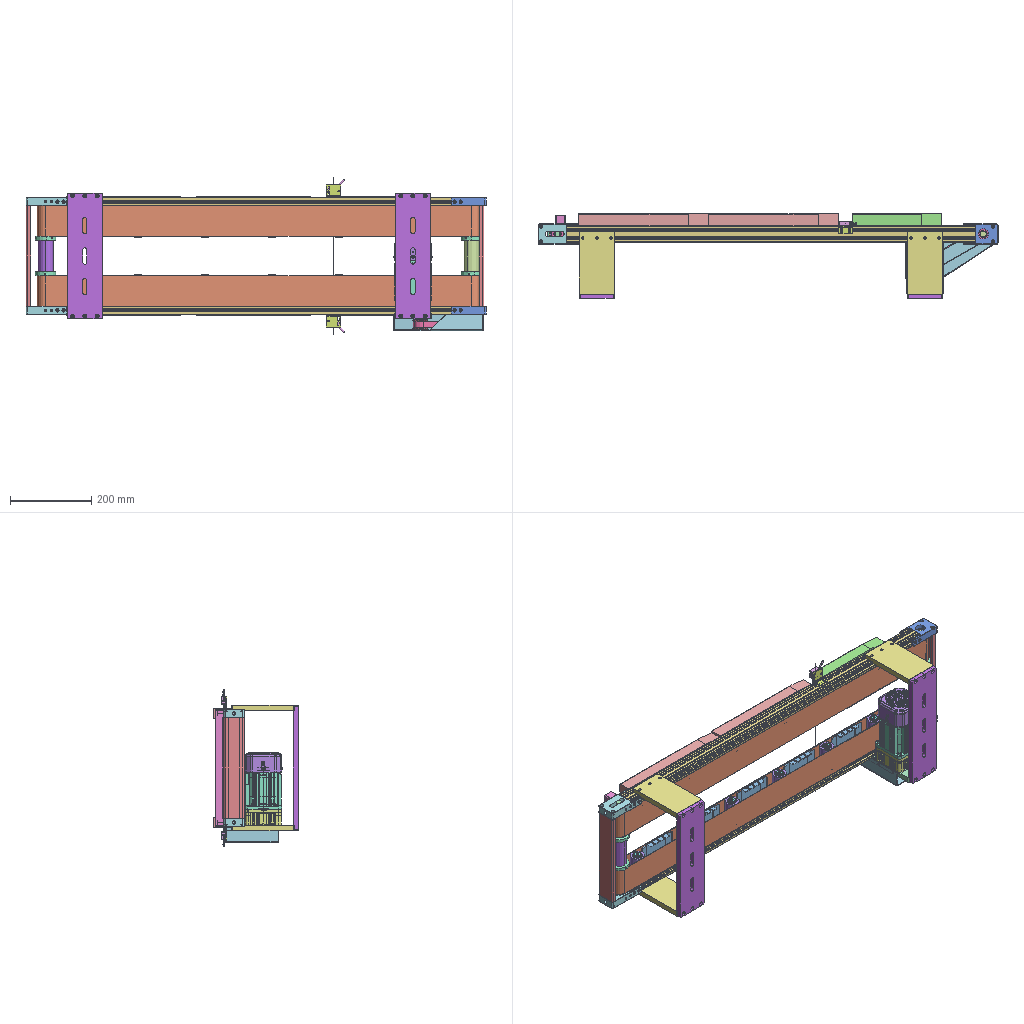Assembly | STEP file | 58 different items | 160 placed | box 1133 x 208 x 386 mm
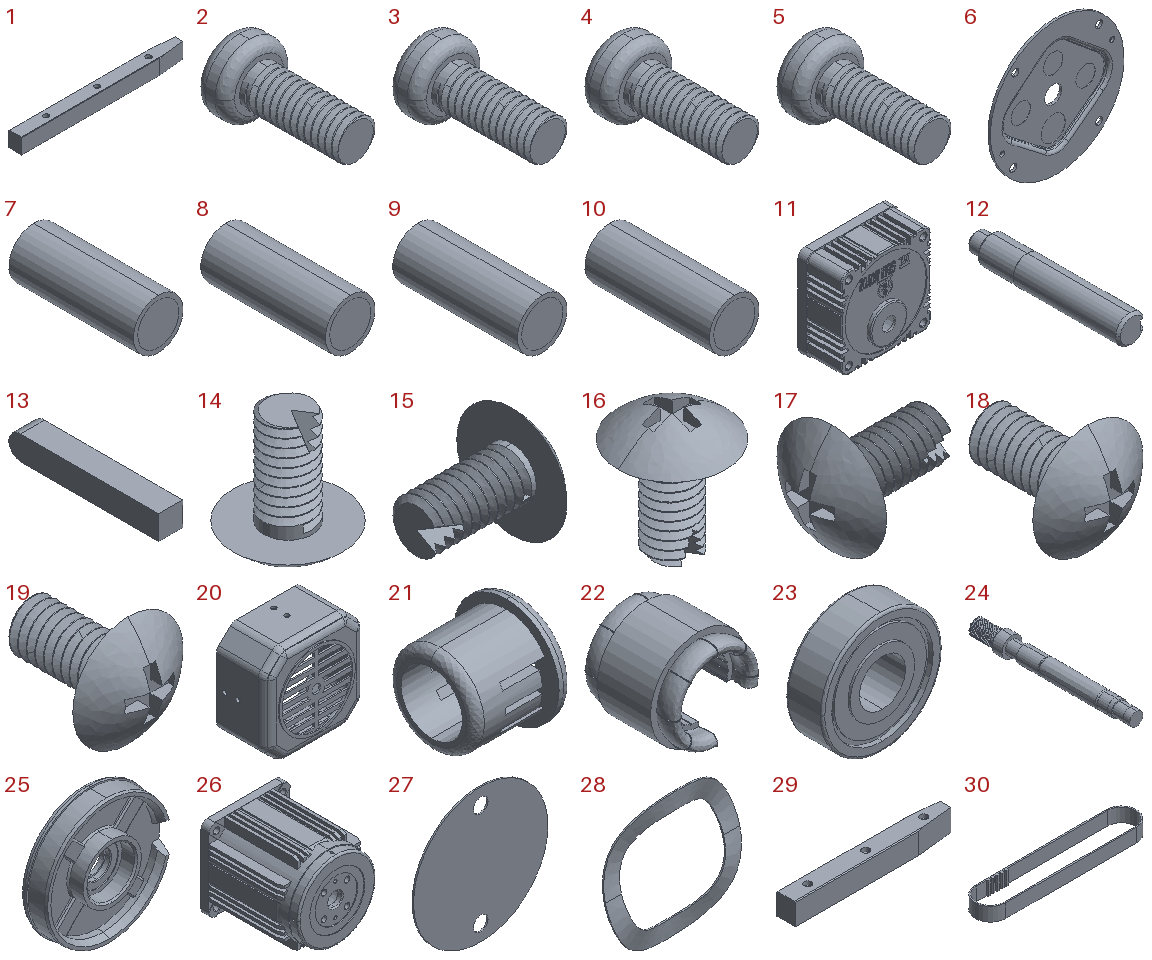Parts list (item | quantity | size | volume):
1 | x4 | 320 x 25 x 30 mm | 229201 mm3
2 | x1 | 7 x 13 x 7 mm | 186.803 mm3
3 | x1 | 7 x 13 x 7 mm | 186.803 mm3
4 | x1 | 7 x 13 x 7 mm | 186.803 mm3
5 | x1 | 7 x 13 x 7 mm | 186.803 mm3
6 | x1 | 82.5 x 4.2 x 82.5 mm | 8185 mm3
7 | x1 | 4 x 10 x 4 mm | 125.664 mm3
8 | x1 | 4 x 10 x 4 mm | 125.664 mm3
9 | x1 | 4 x 10 x 4 mm | 125.664 mm3
10 | x1 | 4 x 10 x 4 mm | 125.664 mm3
11 | x1 | 90 x 45 x 90 mm | 121396 mm3
12 | x1 | 12 x 67 x 12 mm | 6861 mm3
13 | x1 | 4 x 25 x 4 mm | 393.133 mm3
14 | x1 | 9 x 9 x 10.31 mm | 144.628 mm3
15 | x1 | 10.31 x 9 x 9 mm | 144.628 mm3
16 | x1 | 9 x 9 x 10.31 mm | 144.629 mm3
17 | x1 | 10.31 x 9 x 9 mm | 144.629 mm3
18 | x1 | 9 x 10.31 x 9 mm | 144.628 mm3
19 | x1 | 9 x 10.31 x 9 mm | 144.628 mm3
20 | x1 | 90 x 48 x 90 mm | 30003 mm3
21 | x1 | 10 x 12 x 12 mm | 394.73 mm3
22 | x1 | 83 x 81.388 x 83 mm | 169148 mm3
23 | x1 | 26 x 8 x 26 mm | 3318 mm3
24 | x1 | 15 x 120.2 x 15 mm | 12927 mm3
25 | x1 | 85.3 x 18.5 x 85.3 mm | 37197 mm3
26 | x1 | 90 x 106 x 90 mm | 163819 mm3
27 | x1 | 46 x 0.5 x 46 mm | 811.316 mm3
28 | x1 | 25 x 2.25 x 25 mm | 51.836 mm3
29 | x2 | 220 x 25 x 30 mm | 154301 mm3
30 | x1 | 178.871 x 33.871 x 15 mm | 9222 mm3
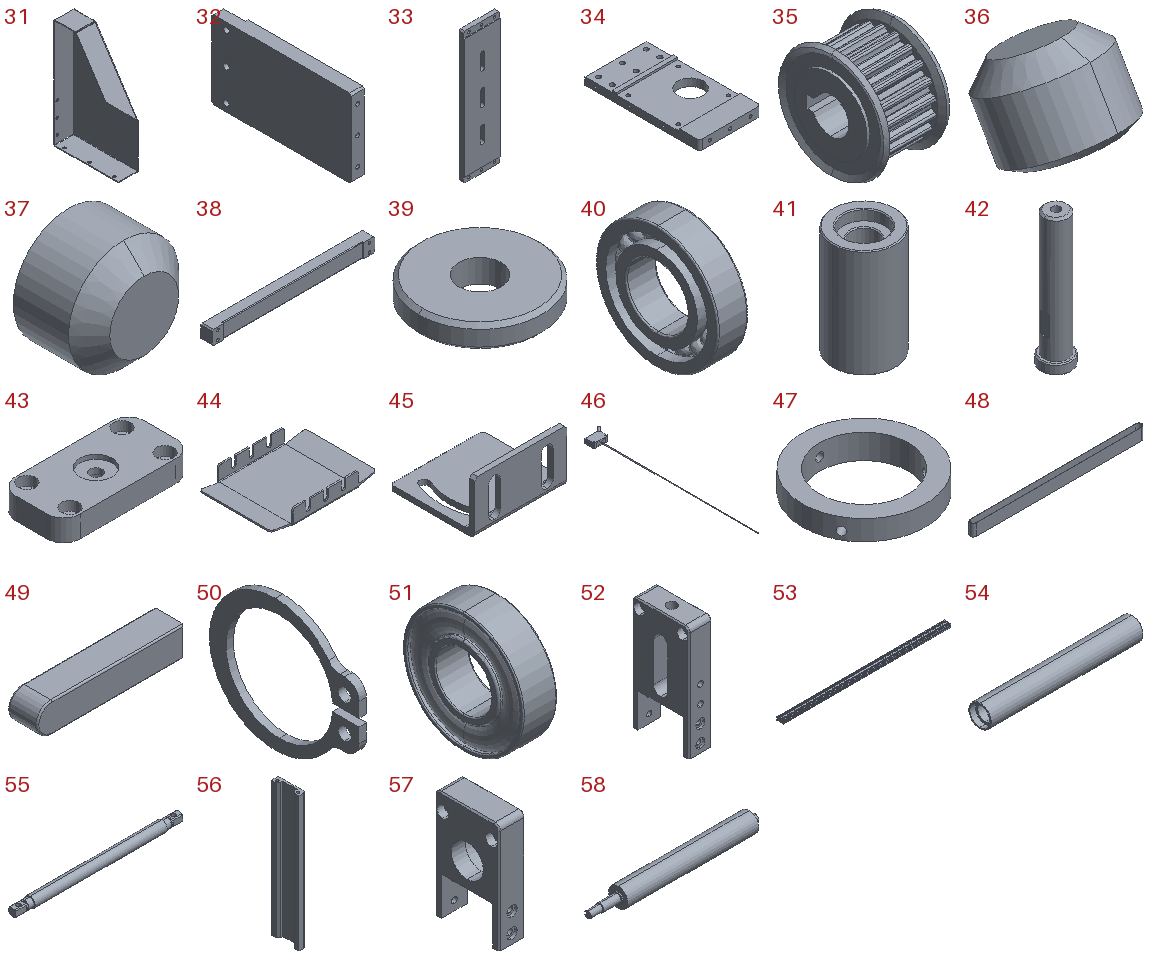31 | x1 | 40 x 130 x 220 mm | 63688 mm3
32 | x3 | 14 x 154 x 86 mm | 176980 mm3
33 | x2 | 86 x 12 x 310 mm | 297335 mm3
34 | x1 | 90 x 168 x 14 mm | 160031 mm3
35 | x2 | 22 x 36 x 36 mm | 12348 mm3
36 | x2 | 4 x 4.465 x 4.008 mm | 28.763 mm3
37 | x2 | 4 x 3 x 4 mm | 28.763 mm3
38 | x1 | 288 x 20 x 25 mm | 129456 mm3
39 | x12 | 16 x 16 x 3 mm | 519.606 mm3
40 | x24 | 6 x 24 x 24 mm | 1508 mm3
41 | x12 | 36 x 36 x 62 mm | 48785 mm3
42 | x12 | 15 x 15 x 67 mm | 7479 mm3
43 | x12 | 60 x 30 x 10 mm | 15370 mm3
44 | x12 | 104.913 x 75 x 15.5 mm | 13779 mm3
45 | x2 | 35 x 32 x 20 mm | 3068 mm3
46 | x2 | 44.556 x 382.556 x 10.8 mm | 7259 mm3
47 | x4 | 50 x 50 x 10 mm | 8609 mm3
48 | x2 | 1089 x 40 x 75 mm | 332607 mm3
49 | x1 | 20 x 4 x 4 mm | 312.344 mm3
50 | x2 | 1 x 20 x 17.6 mm | 97.521 mm3
51 | x4 | 9 x 32 x 32 mm | 5285 mm3
52 | x2 | 20 x 50 x 100 mm | 60104 mm3
53 | x2 | 1008 x 40 x 20 mm | 300919 mm3
54 | x1 | 246 x 36 x 36 mm | 123974 mm3
55 | x1 | 288 x 18 x 18 mm | 66372 mm3
56 | x2 | 12 x 50 x 248 mm | 87500 mm3
57 | x2 | 20 x 50 x 85 mm | 46036 mm3
58 | x1 | 311 x 36 x 36 mm | 259033 mm3
Placements (level | parent | child | x y z in mm | rotation matrix by rows):
1 | subassembly 2 | subassembly 3 | -366.772 85.102 -251.356 | 1 0 0 0 0 1 0 -1 -0
1 | subassembly 2 | subassembly 3 | -366.772 85.102 16.645 | 1 0 0 0 0 1 0 -1 0
1 | subassembly 2 | subassembly 4 | 6.367 92.148 -130.675 | 0 0 -1 1 0 0 0 -1 0
2 | subassembly 4 | subassembly 5 | -99.047 109.68 -0.0 | -1 0 0 0 -1 0 0 0 1
2 | subassembly 4 | subassembly 6 | -99.047 109.68 -0.0 | -1 0 0 0 -1 0 0 0 1
2 | subassembly 4 | subassembly 7 | -99.047 109.68 -0.0 | -1 0 0 0 -1 0 0 0 1
2 | subassembly 4 | subassembly 8 | -99.047 109.68 -0.0 | -1 0 0 0 -1 0 0 0 1
2 | subassembly 4 | subassembly 9 | -99.047 109.68 -0.0 | -1 0 0 0 -1 0 0 0 1
2 | subassembly 4 | subassembly 10 | -99.047 109.68 -0.0 | -1 0 0 0 -1 0 0 0 1
2 | subassembly 4 | subassembly 11 | -99.047 109.68 -0.0 | -1 0 0 0 -1 0 0 0 1
2 | subassembly 4 | subassembly 12 | -99.047 109.68 -0.0 | -1 0 0 0 -1 0 0 0 1
2 | subassembly 4 | subassembly 13 | -99.047 109.68 -0.0 | -1 0 0 0 -1 0 0 0 1
2 | subassembly 4 | subassembly 14 | -99.047 109.68 -0.0 | -1 0 0 0 -1 0 0 0 1
2 | subassembly 4 | subassembly 15 | -99.047 109.68 -0.0 | -1 0 0 0 -1 0 0 0 1
2 | subassembly 4 | subassembly 16 | -99.047 109.68 -0.0 | -1 0 0 0 -1 0 0 0 1
2 | subassembly 4 | subassembly 17 | -99.047 80.68 -0.0 | 1 0 0 0 1 0 0 0 1
2 | subassembly 4 | subassembly 18 | -99.047 80.68 -0.0 | 1 0 0 0 1 0 0 0 1
2 | subassembly 4 | subassembly 19 | -99.047 80.68 -0.0 | 1 0 0 0 1 0 0 0 1
2 | subassembly 4 | subassembly 20 | -99.047 80.68 -0.0 | 1 0 0 0 1 0 0 0 1
2 | subassembly 4 | subassembly 21 | -99.047 80.68 -0.0 | 1 0 0 0 1 0 0 0 1
2 | subassembly 4 | subassembly 22 | -99.047 80.68 -0.0 | 1 0 0 0 1 0 0 0 1
2 | subassembly 4 | subassembly 23 | -99.047 80.68 -0.0 | 1 0 0 0 1 0 0 0 1
2 | subassembly 4 | subassembly 24 | -99.047 80.68 -0.0 | 1 0 0 0 1 0 0 0 1
2 | subassembly 4 | subassembly 25 | -99.047 80.68 -0.0 | 1 0 0 0 1 0 0 0 1
2 | subassembly 4 | subassembly 26 | -99.047 80.68 -0.0 | 1 0 0 0 1 0 0 0 1
2 | subassembly 4 | subassembly 27 | -99.047 80.68 -0.0 | 1 0 0 0 1 0 0 0 1
2 | subassembly 4 | subassembly 28 | -99.047 80.68 -0.0 | 1 0 0 0 1 0 0 0 1
2 | subassembly 4 | subassembly 29 | -99.047 80.68 -0.0 | 1 0 0 0 1 0 0 0 1
2 | subassembly 4 | subassembly 30 | -99.047 80.68 -0.0 | 1 0 0 0 1 0 0 0 1
2 | subassembly 4 | subassembly 31 | -99.047 80.68 -0.0 | 1 0 0 0 1 0 0 0 1
1 | subassembly 2 | subassembly 32 | -61.772 85.102 -251.356 | 1 0 0 0 0 1 0 -1 -0
1 | subassembly 2 | subassembly 32 | -61.772 85.102 16.645 | 1 0 0 0 0 1 0 -1 0
1 | subassembly 2 | subassembly 33 | 24.367 -6.898 -285.356 | 0.868 -0.4966 0 0.4966 0.868 0 0 0 1
1 | subassembly 2 | subassembly 34 | 179.367 86.602 -301.356 | 0 0 1 0 1 0 -1 0 -0
1 | subassembly 2 | subassembly 35 | -36.633 -82.898 37.645 | 0 0 1 0 1 0 -1 0 -0
1 | subassembly 2 | subassembly 36 | 6.367 -87.898 -117.356 | 1 0 0 0 -1 0 0 0 -1
1 | subassembly 2 | subassembly 37 | 6.367 1.102 -272.356 | 1 0 0 0 1 0 0 0 1
1 | subassembly 2 | subassembly 38 | 24.367 -6.898 -296.356 | 0 0 1 0 -1 0 1 0 -0
1 | subassembly 2 | subassembly 39 | 24.367 -6.898 -296.356 | 0 0 1 0 -1 0 1 0 -0
1 | subassembly 2 | subassembly 40 | 24.367 -6.898 -296.356 | 0 0 1 0 -1 0 1 0 -0
1 | subassembly 2 | subassembly 41 | -891.772 90.102 -117.356 | 0 0 1 0 1 0 -1 0 0
1 | subassembly 2 | subassembly 42 | -835.329 65.102 -241.356 | -1 0 0 0 -1 0 0 0 1
2 | subassembly 42 | subassembly 43 | -0.0 0.0 75.0 | 0.997 -0.07694 0 0.07694 0.997 0 0 0 1
2 | subassembly 42 | subassembly 44 | -0.0 0.0 72.0 | 0 0.9146 -0.4044 0 0.4044 0.9146 1 0 -0
2 | subassembly 42 | subassembly 45 | -0.0 0.0 75.0 | 0.626 0.7798 0 0.7798 -0.626 0 0 0 -1
2 | subassembly 42 | subassembly 44 | 0.0 0.0 16.0 | 0 -0.9997 0.02322 0 0.02322 0.9997 -1 0 -0
2 | subassembly 42 | subassembly 46 | 0.0 -0.0 8.0 | 0.2901 0.957 0 -0.957 0.2901 0 0 0 1
2 | subassembly 42 | subassembly 47 | -0.0 -0.0 -0.0 | 1 0 0 0 1 0 0 0 1
1 | subassembly 2 | subassembly 48 | -752.829 81.602 -203.856 | -1 0 0 0 0 -1 0 -1 -0
1 | subassembly 2 | subassembly 49 | -670.329 65.102 -241.356 | -1 0 0 0 -1 0 0 0 1
2 | subassembly 49 | subassembly 43 | -0.0 0.0 75.0 | 0.997 -0.07694 0 0.07694 0.997 0 0 0 1
2 | subassembly 49 | subassembly 44 | -0.0 0.0 72.0 | 0 0.9146 -0.4044 0 0.4044 0.9146 1 0 -0
2 | subassembly 49 | subassembly 45 | -0.0 0.0 75.0 | 0.626 0.7798 0 0.7798 -0.626 0 0 0 -1
2 | subassembly 49 | subassembly 44 | 0.0 0.0 16.0 | 0 -0.9997 0.02322 0 0.02322 0.9997 -1 0 -0
2 | subassembly 49 | subassembly 46 | 0.0 -0.0 8.0 | 0.2901 0.957 0 -0.957 0.2901 0 0 0 1
2 | subassembly 49 | subassembly 47 | -0.0 -0.0 -0.0 | 1 0 0 0 1 0 0 0 1
1 | subassembly 2 | subassembly 48 | -587.829 81.602 -203.856 | -1 0 0 0 0 -1 0 -1 -0
1 | subassembly 2 | subassembly 48 | -422.829 81.602 -203.856 | -1 0 0 0 0 -1 0 -1 -0
1 | subassembly 2 | subassembly 50 | -340.329 65.102 -241.356 | -1 0 0 0 -1 0 0 0 1
2 | subassembly 50 | subassembly 43 | -0.0 0.0 75.0 | 0.997 -0.07694 0 0.07694 0.997 0 0 0 1
2 | subassembly 50 | subassembly 44 | -0.0 0.0 72.0 | 0 0.9146 -0.4044 0 0.4044 0.9146 1 0 -0
2 | subassembly 50 | subassembly 45 | -0.0 0.0 75.0 | 0.626 0.7798 0 0.7798 -0.626 0 0 0 -1
2 | subassembly 50 | subassembly 44 | -0.0 0.0 16.0 | 0 -0.9997 0.02322 0 0.02322 0.9997 -1 0 -0
2 | subassembly 50 | subassembly 46 | 0.0 -0.0 8.0 | 0.2901 0.957 0 -0.957 0.2901 0 0 0 1
2 | subassembly 50 | subassembly 47 | -0.0 -0.0 -0.0 | 1 0 0 0 1 0 0 0 1
1 | subassembly 2 | subassembly 51 | -175.329 65.102 -241.356 | -1 0 0 0 -1 0 0 0 1
2 | subassembly 51 | subassembly 43 | -0.0 0.0 75.0 | 0.997 -0.07694 0 0.07694 0.997 0 0 0 1
2 | subassembly 51 | subassembly 44 | -0.0 0.0 72.0 | 0 0.9146 -0.4044 0 0.4044 0.9146 1 0 -0
2 | subassembly 51 | subassembly 45 | -0.0 0.0 75.0 | 0.626 0.7798 0 0.7798 -0.626 0 0 0 -1
2 | subassembly 51 | subassembly 44 | -0.0 0.0 16.0 | 0 -0.9997 0.02322 0 0.02322 0.9997 -1 0 -0
2 | subassembly 51 | subassembly 46 | 0.0 -0.0 8.0 | 0.2901 0.957 0 -0.957 0.2901 0 0 0 1
2 | subassembly 51 | subassembly 47 | -0.0 -0.0 -0.0 | 1 0 0 0 1 0 0 0 1
1 | subassembly 2 | subassembly 48 | -257.829 81.602 -203.856 | -1 0 0 0 0 -1 0 -1 -0
1 | subassembly 2 | subassembly 48 | 72.171 81.602 -203.856 | -1 0 0 0 0 -1 0 -1 -0
1 | subassembly 2 | subassembly 48 | -92.829 81.602 -203.856 | -1 0 0 0 0 -1 0 -1 -0
1 | subassembly 2 | subassembly 52 | -10.329 65.102 -241.356 | -1 0 0 0 -1 0 0 0 1
2 | subassembly 52 | subassembly 43 | -0.0 0.0 75.0 | 0.997 -0.07694 0 0.07694 0.997 0 0 0 1
2 | subassembly 52 | subassembly 44 | -0.0 0.0 72.0 | 0 0.9146 -0.4044 0 0.4044 0.9146 1 0 -0
2 | subassembly 52 | subassembly 45 | -0.0 0.0 75.0 | 0.626 0.7798 0 0.7798 -0.626 0 0 0 -1
2 | subassembly 52 | subassembly 44 | -0.0 0.0 16.0 | 0 -0.9997 0.02322 0 0.02322 0.9997 -1 0 -0
2 | subassembly 52 | subassembly 46 | 0.0 -0.0 8.0 | 0.2901 0.957 0 -0.957 0.2901 0 0 0 1
2 | subassembly 52 | subassembly 47 | -0.0 -0.0 -0.0 | 1 0 0 0 1 0 0 0 1
1 | subassembly 2 | subassembly 53 | -505.329 65.102 -241.356 | -1 0 0 0 -1 0 0 0 1
2 | subassembly 53 | subassembly 43 | -0.0 0.0 75.0 | 0.997 -0.07694 0 0.07694 0.997 0 0 0 1
2 | subassembly 53 | subassembly 44 | -0.0 0.0 72.0 | 0 0.9146 -0.4044 0 0.4044 0.9146 1 0 -0
2 | subassembly 53 | subassembly 45 | -0.0 0.0 75.0 | 0.626 0.7798 0 0.7798 -0.626 0 0 0 -1
2 | subassembly 53 | subassembly 44 | 0.0 0.0 16.0 | 0 -0.9997 0.02322 0 0.02322 0.9997 -1 0 -0
2 | subassembly 53 | subassembly 46 | 0.0 -0.0 8.0 | 0.2901 0.957 0 -0.957 0.2901 0 0 0 1
2 | subassembly 53 | subassembly 47 | -0.0 -0.0 -0.0 | 1 0 0 0 1 0 0 0 1
1 | subassembly 2 | subassembly 38 | 150.228 65.102 -296.356 | 0 -0.8048 -0.5935 0 0.5935 -0.8048 1 0 0
1 | subassembly 2 | subassembly 39 | 150.228 65.102 -296.356 | 0 -0.8048 -0.5935 0 0.5935 -0.8048 1 0 0
1 | subassembly 2 | subassembly 40 | 150.228 65.102 -296.356 | 0 -0.8048 -0.5935 0 0.5935 -0.8048 1 0 0
1 | subassembly 2 | subassembly 48 | -752.829 81.602 -30.855 | 1 0 0 0 0 -1 0 1 0
1 | subassembly 2 | subassembly 54 | -835.329 65.102 6.644 | -1 0 0 0 1 0 0 0 -1
2 | subassembly 54 | subassembly 43 | -0.0 0.0 75.0 | 0.997 -0.07694 0 0.07694 0.997 0 0 0 1
2 | subassembly 54 | subassembly 44 | -0.0 0.0 72.0 | 0 0.9146 -0.4044 0 0.4044 0.9146 1 0 -0
2 | subassembly 54 | subassembly 45 | -0.0 0.0 75.0 | 0.626 0.7798 0 0.7798 -0.626 0 0 0 -1
2 | subassembly 54 | subassembly 44 | 0.0 0.0 16.0 | 0 -0.9997 0.02322 0 0.02322 0.9997 -1 0 -0
2 | subassembly 54 | subassembly 46 | 0.0 -0.0 8.0 | 0.2901 0.957 0 -0.957 0.2901 0 0 0 1
2 | subassembly 54 | subassembly 47 | -0.0 -0.0 -0.0 | 1 0 0 0 1 0 0 0 1
1 | subassembly 2 | subassembly 55 | -670.329 65.102 6.644 | -1 0 0 0 1 0 0 0 -1
2 | subassembly 55 | subassembly 43 | -0.0 0.0 75.0 | 0.997 -0.07694 0 0.07694 0.997 0 0 0 1
2 | subassembly 55 | subassembly 44 | -0.0 0.0 72.0 | 0 0.9146 -0.4044 0 0.4044 0.9146 1 0 -0
2 | subassembly 55 | subassembly 45 | -0.0 0.0 75.0 | 0.626 0.7798 0 0.7798 -0.626 0 0 0 -1
2 | subassembly 55 | subassembly 44 | 0.0 0.0 16.0 | 0 -0.9997 0.02322 0 0.02322 0.9997 -1 0 -0
2 | subassembly 55 | subassembly 46 | 0.0 -0.0 8.0 | 0.2901 0.957 0 -0.957 0.2901 0 0 0 1
2 | subassembly 55 | subassembly 47 | -0.0 -0.0 -0.0 | 1 0 0 0 1 0 0 0 1
1 | subassembly 2 | subassembly 48 | -587.829 81.602 -30.855 | 1 0 0 0 0 -1 0 1 0
1 | subassembly 2 | subassembly 56 | -189.272 75.102 26.645 | 1 0 0 0 0 -1 0 1 0
1 | subassembly 2 | subassembly 56 | -189.272 75.102 -261.356 | -1 0 0 0 0 -1 0 -1 -0
1 | subassembly 2 | subassembly 57 | -189.272 90.502 -274.356 | 1 0 0 0 0 1 0 -1 0
1 | subassembly 2 | subassembly 57 | -189.272 90.502 39.645 | 1 0 0 0 0 -1 0 1 -0
1 | subassembly 2 | subassembly 58 | -505.329 65.102 6.644 | -1 0 0 0 1 0 0 0 -1
2 | subassembly 58 | subassembly 43 | -0.0 0.0 75.0 | 0.997 -0.07694 0 0.07694 0.997 0 0 0 1
2 | subassembly 58 | subassembly 44 | -0.0 0.0 72.0 | 0 0.9146 -0.4044 0 0.4044 0.9146 1 0 -0
2 | subassembly 58 | subassembly 45 | -0.0 0.0 75.0 | 0.626 0.7798 0 0.7798 -0.626 0 0 0 -1
2 | subassembly 58 | subassembly 44 | 0.0 0.0 16.0 | 0 -0.9997 0.02322 0 0.02322 0.9997 -1 0 -0
2 | subassembly 58 | subassembly 46 | 0.0 -0.0 8.0 | 0.2901 0.957 0 -0.957 0.2901 0 0 0 1
2 | subassembly 58 | subassembly 47 | -0.0 -0.0 -0.0 | 1 0 0 0 1 0 0 0 1
1 | subassembly 2 | subassembly 59 | -340.329 65.102 6.644 | -1 0 0 0 1 0 0 0 -1
2 | subassembly 59 | subassembly 43 | -0.0 0.0 75.0 | 0.997 -0.07694 0 0.07694 0.997 0 0 0 1
2 | subassembly 59 | subassembly 44 | -0.0 0.0 72.0 | 0 0.9146 -0.4044 0 0.4044 0.9146 1 0 -0
2 | subassembly 59 | subassembly 45 | -0.0 0.0 75.0 | 0.626 0.7798 0 0.7798 -0.626 0 0 0 -1
2 | subassembly 59 | subassembly 44 | -0.0 0.0 16.0 | 0 -0.9997 0.02322 0 0.02322 0.9997 -1 0 -0
2 | subassembly 59 | subassembly 46 | 0.0 -0.0 8.0 | 0.2901 0.957 0 -0.957 0.2901 0 0 0 1
2 | subassembly 59 | subassembly 47 | -0.0 -0.0 -0.0 | 1 0 0 0 1 0 0 0 1
1 | subassembly 2 | subassembly 60 | -175.329 65.102 6.644 | -1 0 0 0 1 0 0 0 -1
2 | subassembly 60 | subassembly 43 | -0.0 0.0 75.0 | 0.997 -0.07694 0 0.07694 0.997 0 0 0 1
2 | subassembly 60 | subassembly 44 | -0.0 0.0 72.0 | 0 0.9146 -0.4044 0 0.4044 0.9146 1 0 -0
2 | subassembly 60 | subassembly 45 | -0.0 0.0 75.0 | 0.626 0.7798 0 0.7798 -0.626 0 0 0 -1
2 | subassembly 60 | subassembly 44 | -0.0 0.0 16.0 | 0 -0.9997 0.02322 0 0.02322 0.9997 -1 0 -0
2 | subassembly 60 | subassembly 46 | 0.0 -0.0 8.0 | 0.2901 0.957 0 -0.957 0.2901 0 0 0 1
2 | subassembly 60 | subassembly 47 | -0.0 -0.0 -0.0 | 1 0 0 0 1 0 0 0 1
1 | subassembly 2 | subassembly 48 | -422.829 81.602 -30.855 | 1 0 0 0 0 -1 0 1 0
1 | subassembly 2 | subassembly 48 | -257.829 81.602 -30.855 | 1 0 0 0 0 -1 0 1 0
1 | subassembly 2 | subassembly 48 | -92.829 81.602 -30.855 | 1 0 0 0 0 -1 0 1 0
1 | subassembly 2 | subassembly 61 | -10.329 65.102 6.644 | -1 0 0 0 1 0 0 0 -1
2 | subassembly 61 | subassembly 43 | -0.0 0.0 75.0 | 0.997 -0.07694 0 0.07694 0.997 0 0 0 1
2 | subassembly 61 | subassembly 44 | -0.0 0.0 72.0 | 0 0.9146 -0.4044 0 0.4044 0.9146 1 0 -0
2 | subassembly 61 | subassembly 45 | -0.0 0.0 75.0 | 0.626 0.7798 0 0.7798 -0.626 0 0 0 -1
2 | subassembly 61 | subassembly 44 | -0.0 0.0 16.0 | 0 -0.9997 0.02322 0 0.02322 0.9997 -1 0 -0
2 | subassembly 61 | subassembly 46 | 0.0 -0.0 8.0 | 0.2901 0.957 0 -0.957 0.2901 0 0 0 1
2 | subassembly 61 | subassembly 47 | -0.0 -0.0 -0.0 | 1 0 0 0 1 0 0 0 1
1 | subassembly 2 | subassembly 62 | 150.228 65.102 -166.356 | 0.2927 0.9562 0 -0.9562 0.2927 0 0 0 1
1 | subassembly 2 | subassembly 62 | 150.228 65.102 -68.356 | 0.008437 1 0 1 -0.008437 0 0 0 -1
1 | subassembly 2 | subassembly 62 | -898.772 65.102 -166.356 | -0.9995 -0.03158 0 0.03158 -0.9995 0 0 0 1
1 | subassembly 2 | subassembly 62 | -898.772 65.102 -68.356 | 0.1258 -0.9921 0 -0.9921 -0.1258 0 0 0 -1
1 | subassembly 2 | subassembly 63 | 150.228 65.102 -30.855 | 1 0 0 0 1 0 0 0 1
1 | subassembly 2 | subassembly 64 | 145.801 68.366 -277.356 | 0 -0.8048 0.5935 0 0.5935 0.8048 -1 0 -0
1 | subassembly 2 | subassembly 65 | -898.772 65.102 6.144 | 0 0 1 0 1 0 -1 0 -0
1 | subassembly 2 | subassembly 65 | -898.772 65.102 -240.856 | 0 0 1 0 1 0 -1 0 -0
1 | subassembly 2 | subassembly 66 | 150.228 65.102 -241.356 | 0 0.1138 0.9935 0 0.9935 -0.1138 -1 0 -0
1 | subassembly 2 | subassembly 66 | 150.228 65.102 15.645 | 0 -0.6117 -0.7911 0 -0.7911 0.6117 -1 0 0
1 | subassembly 2 | subassembly 66 | -898.772 65.102 -231.356 | 0 -0.6802 -0.733 0 -0.733 0.6802 -1 0 0
1 | subassembly 2 | subassembly 66 | -898.772 65.102 5.644 | 0 0.552 0.8339 0 0.8339 -0.552 -1 0 -0
1 | subassembly 2 | subassembly 67 | -896.772 65.102 26.645 | 0 0 -1 0 -1 0 -1 0 0
1 | subassembly 2 | subassembly 67 | -896.772 65.102 -261.356 | 0 0 -1 0 1 0 1 0 0
1 | subassembly 2 | subassembly 63 | 150.228 65.102 -203.856 | 1 0 0 0 1 0 0 0 1
1 | subassembly 2 | subassembly 35 | -844.772 -82.898 37.645 | 0 0 1 0 1 0 -1 0 -0
1 | subassembly 2 | subassembly 35 | -758.772 -82.898 -272.356 | 0 0 -1 0 1 0 1 0 0
1 | subassembly 2 | subassembly 36 | -801.772 -87.898 -117.356 | 1 0 0 0 -1 0 0 0 -1
1 | subassembly 2 | subassembly 48 | 72.171 81.602 -30.855 | 1 0 0 0 0 -1 0 1 0
1 | subassembly 2 | subassembly 3 | -686.772 85.102 -251.356 | 1 0 0 0 0 1 0 -1 -0
1 | subassembly 2 | subassembly 3 | -686.772 85.102 16.645 | 1 0 0 0 0 1 0 -1 0
1 | subassembly 2 | subassembly 68 | -372.772 65.102 -251.356 | 1 0 0 0 1 0 0 0 1
1 | subassembly 2 | subassembly 68 | -372.772 65.102 16.645 | 1 0 0 0 1 0 0 0 1
1 | subassembly 2 | subassembly 69 | -898.772 65.102 -117.356 | 0 -0.9999 -0.0167 0 0.0167 -0.9999 1 0 0
1 | subassembly 2 | subassembly 70 | -898.772 65.102 -117.356 | 0 0 -1 0 1 0 1 0 0
1 | subassembly 2 | subassembly 71 | -934.772 65.102 -117.356 | -1 0 0 0 -1 0 0 0 1
1 | subassembly 2 | subassembly 71 | 169.228 65.102 -117.356 | 1 0 0 0 -1 0 0 0 -1
1 | subassembly 2 | subassembly 72 | 143.728 65.102 -261.356 | 0 0 1 0 -1 0 1 0 -0
1 | subassembly 2 | subassembly 72 | 143.728 65.102 26.645 | 0 0 1 0 1 0 -1 0 0
1 | subassembly 2 | subassembly 73 | 150.228 65.102 -295.356 | 0 -0.8048 -0.5935 0 0.5935 -0.8048 1 0 0